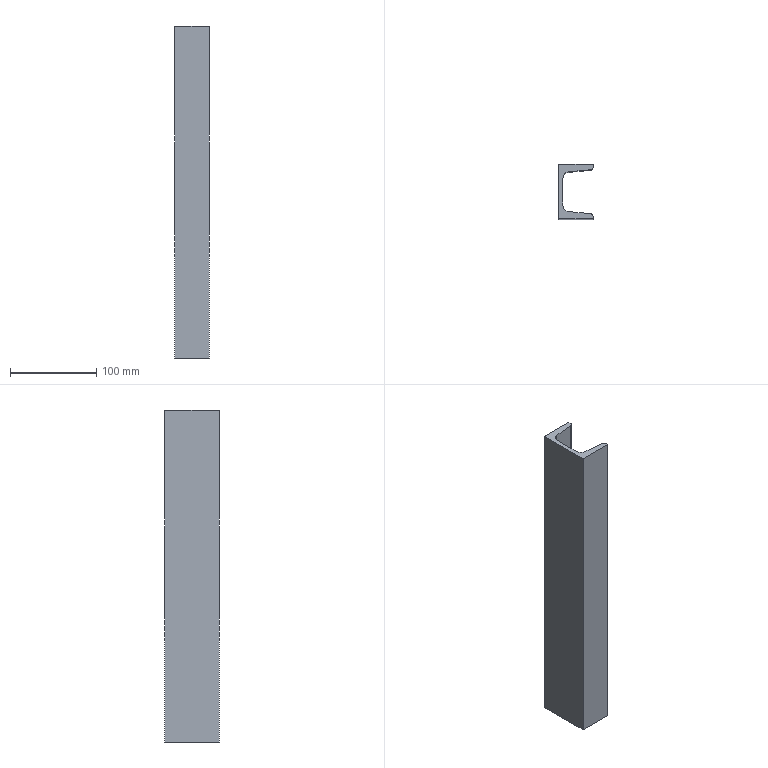Part | STEP file | 750038229 | 1 solid | 14 faces | box 40 x 63 x 384 mm | volume 324314 mm3 | plane 10 | cylinder 4 | commonest cylinder face diameters 7.6 x2 15 x2
STEP:
#1=CARTESIAN_POINT('',(0.,0.,192.));
#2=VERTEX_POINT('',#1);
#3=CARTESIAN_POINT('',(0.,0.,-192.));
#4=VERTEX_POINT('',#3);
#5=CARTESIAN_POINT('',(0.,0.,192.));
#6=DIRECTION('',(0.,0.,-1.));
#7=VECTOR('',#6,1000.);
#8=LINE('',#5,#7);
#9=EDGE_CURVE('',#2,#4,#8,.T.);
#10=ORIENTED_EDGE('',*,*,#9,.F.);
#11=CARTESIAN_POINT('',(0.,63.,192.));
#12=VERTEX_POINT('',#11);
#13=CARTESIAN_POINT('',(0.,63.,192.));
#14=DIRECTION('',(0.,-1.,0.));
#15=VECTOR('',#14,1000.);
#16=LINE('',#13,#15);
#17=EDGE_CURVE('',#12,#2,#16,.T.);
#18=ORIENTED_EDGE('',*,*,#17,.F.);
#19=CARTESIAN_POINT('',(0.,63.,-192.));
#20=VERTEX_POINT('',#19);
#21=CARTESIAN_POINT('',(0.,63.,192.));
#22=DIRECTION('',(0.,0.,1.));
#23=VECTOR('',#22,1000.);
#24=LINE('',#21,#23);
#25=EDGE_CURVE('',#20,#12,#24,.T.);
#26=ORIENTED_EDGE('',*,*,#25,.F.);
#27=CARTESIAN_POINT('',(0.,63.,-192.));
#28=DIRECTION('',(0.,1.,0.));
#29=VECTOR('',#28,1000.);
#30=LINE('',#27,#29);
#31=EDGE_CURVE('',#4,#20,#30,.T.);
#32=ORIENTED_EDGE('',*,*,#31,.F.);
#33=EDGE_LOOP('',(#10,#18,#26,#32));
#34=FACE_OUTER_BOUND('',#33,.T.);
#35=CARTESIAN_POINT('',(0.,63.,192.));
#36=DIRECTION('',(1.,0.,0.));
#37=DIRECTION('',(0.,0.,-1.));
#38=AXIS2_PLACEMENT_3D('',#35,#36,#37);
#39=PLANE('',#38);
#40=ADVANCED_FACE('',(#34),#39,.F.);
#41=CARTESIAN_POINT('',(40.,63.,-192.));
#42=VERTEX_POINT('',#41);
#43=CARTESIAN_POINT('',(36.2,63.,-192.));
#44=DIRECTION('',(-1.,0.,0.));
#45=VECTOR('',#44,1000.);
#46=LINE('',#43,#45);
#47=EDGE_CURVE('',#42,#20,#46,.T.);
#48=ORIENTED_EDGE('',*,*,#47,.F.);
#49=CARTESIAN_POINT('',(40.,60.699,-192.));
#50=VERTEX_POINT('',#49);
#51=CARTESIAN_POINT('',(40.,2.301,-192.));
#52=DIRECTION('',(0.,1.,0.));
#53=VECTOR('',#52,1000.);
#54=LINE('',#51,#53);
#55=EDGE_CURVE('',#50,#42,#54,.T.);
#56=ORIENTED_EDGE('',*,*,#55,.F.);
#57=CARTESIAN_POINT('',(36.578,56.918,-192.));
#58=VERTEX_POINT('',#57);
#59=CARTESIAN_POINT('',(36.2,60.699,-192.));
#60=DIRECTION('',(0.,0.,1.));
#61=DIRECTION('',(-1.,0.,0.));
#62=AXIS2_PLACEMENT_3D('',#59,#60,#61);
#63=CIRCLE('',#62,3.8);
#64=EDGE_CURVE('',#58,#50,#63,.T.);
#65=ORIENTED_EDGE('',*,*,#64,.F.);
#66=CARTESIAN_POINT('',(11.554,54.415,-192.));
#67=VERTEX_POINT('',#66);
#68=CARTESIAN_POINT('',(11.554,54.415,-192.));
#69=DIRECTION('',(0.995,0.0995,0.));
#70=VECTOR('',#69,1000.);
#71=LINE('',#68,#70);
#72=EDGE_CURVE('',#67,#58,#71,.T.);
#73=ORIENTED_EDGE('',*,*,#72,.F.);
#74=CARTESIAN_POINT('',(4.8,46.953,-192.));
#75=VERTEX_POINT('',#74);
#76=CARTESIAN_POINT('',(12.3,46.953,-192.));
#77=DIRECTION('',(0.,0.,-1.));
#78=DIRECTION('',(-1.,0.,0.));
#79=AXIS2_PLACEMENT_3D('',#76,#77,#78);
#80=CIRCLE('',#79,7.5);
#81=EDGE_CURVE('',#75,#67,#80,.T.);
#82=ORIENTED_EDGE('',*,*,#81,.F.);
#83=CARTESIAN_POINT('',(4.8,16.047,-192.));
#84=VERTEX_POINT('',#83);
#85=CARTESIAN_POINT('',(4.8,2.301,-192.));
#86=DIRECTION('',(0.,1.,0.));
#87=VECTOR('',#86,1000.);
#88=LINE('',#85,#87);
#89=EDGE_CURVE('',#84,#75,#88,.T.);
#90=ORIENTED_EDGE('',*,*,#89,.F.);
#91=CARTESIAN_POINT('',(11.554,8.585,-192.));
#92=VERTEX_POINT('',#91);
#93=CARTESIAN_POINT('',(12.3,16.047,-192.));
#94=DIRECTION('',(0.,0.,-1.));
#95=DIRECTION('',(-1.,0.,0.));
#96=AXIS2_PLACEMENT_3D('',#93,#94,#95);
#97=CIRCLE('',#96,7.5);
#98=EDGE_CURVE('',#92,#84,#97,.T.);
#99=ORIENTED_EDGE('',*,*,#98,.F.);
#100=CARTESIAN_POINT('',(36.578,6.082,-192.));
#101=VERTEX_POINT('',#100);
#102=CARTESIAN_POINT('',(36.578,6.082,-192.));
#103=DIRECTION('',(-0.995,0.0995,0.));
#104=VECTOR('',#103,1000.);
#105=LINE('',#102,#104);
#106=EDGE_CURVE('',#101,#92,#105,.T.);
#107=ORIENTED_EDGE('',*,*,#106,.F.);
#108=CARTESIAN_POINT('',(40.,2.301,-192.));
#109=VERTEX_POINT('',#108);
#110=CARTESIAN_POINT('',(36.2,2.301,-192.));
#111=DIRECTION('',(0.,0.,1.));
#112=DIRECTION('',(-1.,0.,0.));
#113=AXIS2_PLACEMENT_3D('',#110,#111,#112);
#114=CIRCLE('',#113,3.8);
#115=EDGE_CURVE('',#109,#101,#114,.T.);
#116=ORIENTED_EDGE('',*,*,#115,.F.);
#117=CARTESIAN_POINT('',(40.,0.,-192.));
#118=VERTEX_POINT('',#117);
#119=CARTESIAN_POINT('',(40.,2.301,-192.));
#120=DIRECTION('',(0.,1.,0.));
#121=VECTOR('',#120,1000.);
#122=LINE('',#119,#121);
#123=EDGE_CURVE('',#118,#109,#122,.T.);
#124=ORIENTED_EDGE('',*,*,#123,.F.);
#125=CARTESIAN_POINT('',(36.2,0.,-192.));
#126=DIRECTION('',(1.,0.,0.));
#127=VECTOR('',#126,1000.);
#128=LINE('',#125,#127);
#129=EDGE_CURVE('',#4,#118,#128,.T.);
#130=ORIENTED_EDGE('',*,*,#129,.F.);
#131=ORIENTED_EDGE('',*,*,#31,.T.);
#132=EDGE_LOOP('',(#48,#56,#65,#73,#82,#90,#99,#107,#116,#124,#130,#131));
#133=FACE_OUTER_BOUND('',#132,.T.);
#134=CARTESIAN_POINT('',(36.2,2.301,-192.));
#135=DIRECTION('',(0.,0.,1.));
#136=DIRECTION('',(1.,0.,0.));
#137=AXIS2_PLACEMENT_3D('',#134,#135,#136);
#138=PLANE('',#137);
#139=ADVANCED_FACE('',(#133),#138,.F.);
#140=CARTESIAN_POINT('',(40.,0.,192.));
#141=VERTEX_POINT('',#140);
#142=CARTESIAN_POINT('',(40.,0.,192.));
#143=DIRECTION('',(0.,0.,-1.));
#144=VECTOR('',#143,1000.);
#145=LINE('',#142,#144);
#146=EDGE_CURVE('',#141,#118,#145,.T.);
#147=ORIENTED_EDGE('',*,*,#146,.F.);
#148=CARTESIAN_POINT('',(0.,0.,192.));
#149=DIRECTION('',(1.,0.,0.));
#150=VECTOR('',#149,1000.);
#151=LINE('',#148,#150);
#152=EDGE_CURVE('',#2,#141,#151,.T.);
#153=ORIENTED_EDGE('',*,*,#152,.F.);
#154=ORIENTED_EDGE('',*,*,#9,.T.);
#155=ORIENTED_EDGE('',*,*,#129,.T.);
#156=EDGE_LOOP('',(#147,#153,#154,#155));
#157=FACE_OUTER_BOUND('',#156,.T.);
#158=CARTESIAN_POINT('',(0.,0.,192.));
#159=DIRECTION('',(0.,1.,0.));
#160=DIRECTION('',(0.,0.,1.));
#161=AXIS2_PLACEMENT_3D('',#158,#159,#160);
#162=PLANE('',#161);
#163=ADVANCED_FACE('',(#157),#162,.F.);
#164=CARTESIAN_POINT('',(40.,60.699,192.));
#165=VERTEX_POINT('',#164);
#166=CARTESIAN_POINT('',(40.,63.,192.));
#167=VERTEX_POINT('',#166);
#168=CARTESIAN_POINT('',(40.,2.301,192.));
#169=DIRECTION('',(0.,1.,0.));
#170=VECTOR('',#169,1000.);
#171=LINE('',#168,#170);
#172=EDGE_CURVE('',#165,#167,#171,.T.);
#173=ORIENTED_EDGE('',*,*,#172,.T.);
#174=CARTESIAN_POINT('',(36.2,63.,192.));
#175=DIRECTION('',(-1.,0.,0.));
#176=VECTOR('',#175,1000.);
#177=LINE('',#174,#176);
#178=EDGE_CURVE('',#167,#12,#177,.T.);
#179=ORIENTED_EDGE('',*,*,#178,.T.);
#180=ORIENTED_EDGE('',*,*,#17,.T.);
#181=ORIENTED_EDGE('',*,*,#152,.T.);
#182=CARTESIAN_POINT('',(40.,2.301,192.));
#183=VERTEX_POINT('',#182);
#184=CARTESIAN_POINT('',(40.,2.301,192.));
#185=DIRECTION('',(0.,1.,0.));
#186=VECTOR('',#185,1000.);
#187=LINE('',#184,#186);
#188=EDGE_CURVE('',#141,#183,#187,.T.);
#189=ORIENTED_EDGE('',*,*,#188,.T.);
#190=CARTESIAN_POINT('',(36.578,6.082,192.));
#191=VERTEX_POINT('',#190);
#192=CARTESIAN_POINT('',(36.2,2.301,192.));
#193=DIRECTION('',(0.,0.,1.));
#194=DIRECTION('',(-1.,0.,0.));
#195=AXIS2_PLACEMENT_3D('',#192,#193,#194);
#196=CIRCLE('',#195,3.8);
#197=EDGE_CURVE('',#183,#191,#196,.T.);
#198=ORIENTED_EDGE('',*,*,#197,.T.);
#199=CARTESIAN_POINT('',(11.554,8.585,192.));
#200=VERTEX_POINT('',#199);
#201=CARTESIAN_POINT('',(36.578,6.082,192.));
#202=DIRECTION('',(-0.995,0.0995,0.));
#203=VECTOR('',#202,1000.);
#204=LINE('',#201,#203);
#205=EDGE_CURVE('',#191,#200,#204,.T.);
#206=ORIENTED_EDGE('',*,*,#205,.T.);
#207=CARTESIAN_POINT('',(4.8,16.047,192.));
#208=VERTEX_POINT('',#207);
#209=CARTESIAN_POINT('',(12.3,16.047,192.));
#210=DIRECTION('',(0.,0.,-1.));
#211=DIRECTION('',(-1.,0.,0.));
#212=AXIS2_PLACEMENT_3D('',#209,#210,#211);
#213=CIRCLE('',#212,7.5);
#214=EDGE_CURVE('',#200,#208,#213,.T.);
#215=ORIENTED_EDGE('',*,*,#214,.T.);
#216=CARTESIAN_POINT('',(4.8,46.953,192.));
#217=VERTEX_POINT('',#216);
#218=CARTESIAN_POINT('',(4.8,2.301,192.));
#219=DIRECTION('',(0.,1.,0.));
#220=VECTOR('',#219,1000.);
#221=LINE('',#218,#220);
#222=EDGE_CURVE('',#208,#217,#221,.T.);
#223=ORIENTED_EDGE('',*,*,#222,.T.);
#224=CARTESIAN_POINT('',(11.554,54.415,192.));
#225=VERTEX_POINT('',#224);
#226=CARTESIAN_POINT('',(12.3,46.953,192.));
#227=DIRECTION('',(0.,0.,-1.));
#228=DIRECTION('',(-1.,0.,0.));
#229=AXIS2_PLACEMENT_3D('',#226,#227,#228);
#230=CIRCLE('',#229,7.5);
#231=EDGE_CURVE('',#217,#225,#230,.T.);
#232=ORIENTED_EDGE('',*,*,#231,.T.);
#233=CARTESIAN_POINT('',(36.578,56.918,192.));
#234=VERTEX_POINT('',#233);
#235=CARTESIAN_POINT('',(11.554,54.415,192.));
#236=DIRECTION('',(0.995,0.0995,0.));
#237=VECTOR('',#236,1000.);
#238=LINE('',#235,#237);
#239=EDGE_CURVE('',#225,#234,#238,.T.);
#240=ORIENTED_EDGE('',*,*,#239,.T.);
#241=CARTESIAN_POINT('',(36.2,60.699,192.));
#242=DIRECTION('',(0.,0.,1.));
#243=DIRECTION('',(-1.,0.,0.));
#244=AXIS2_PLACEMENT_3D('',#241,#242,#243);
#245=CIRCLE('',#244,3.8);
#246=EDGE_CURVE('',#234,#165,#245,.T.);
#247=ORIENTED_EDGE('',*,*,#246,.T.);
#248=EDGE_LOOP('',(#173,#179,#180,#181,#189,#198,#206,#215,#223,#232,#240,#247));
#249=FACE_OUTER_BOUND('',#248,.T.);
#250=CARTESIAN_POINT('',(36.2,2.301,192.));
#251=DIRECTION('',(0.,0.,1.));
#252=DIRECTION('',(1.,0.,0.));
#253=AXIS2_PLACEMENT_3D('',#250,#251,#252);
#254=PLANE('',#253);
#255=ADVANCED_FACE('',(#249),#254,.T.);
#256=ORIENTED_EDGE('',*,*,#25,.T.);
#257=ORIENTED_EDGE('',*,*,#178,.F.);
#258=CARTESIAN_POINT('',(40.,63.,192.));
#259=DIRECTION('',(0.,0.,1.));
#260=VECTOR('',#259,1000.);
#261=LINE('',#258,#260);
#262=EDGE_CURVE('',#42,#167,#261,.T.);
#263=ORIENTED_EDGE('',*,*,#262,.F.);
#264=ORIENTED_EDGE('',*,*,#47,.T.);
#265=EDGE_LOOP('',(#256,#257,#263,#264));
#266=FACE_OUTER_BOUND('',#265,.T.);
#267=CARTESIAN_POINT('',(40.,63.,192.));
#268=DIRECTION('',(0.,-1.,0.));
#269=DIRECTION('',(0.,0.,-1.));
#270=AXIS2_PLACEMENT_3D('',#267,#268,#269);
#271=PLANE('',#270);
#272=ADVANCED_FACE('',(#266),#271,.F.);
#273=ORIENTED_EDGE('',*,*,#262,.T.);
#274=ORIENTED_EDGE('',*,*,#172,.F.);
#275=CARTESIAN_POINT('',(40.,60.699,192.));
#276=DIRECTION('',(0.,0.,1.));
#277=VECTOR('',#276,1000.);
#278=LINE('',#275,#277);
#279=EDGE_CURVE('',#50,#165,#278,.T.);
#280=ORIENTED_EDGE('',*,*,#279,.F.);
#281=ORIENTED_EDGE('',*,*,#55,.T.);
#282=EDGE_LOOP('',(#273,#274,#280,#281));
#283=FACE_OUTER_BOUND('',#282,.T.);
#284=CARTESIAN_POINT('',(40.,60.699,192.));
#285=DIRECTION('',(-1.,0.,0.));
#286=DIRECTION('',(0.,-1.,0.));
#287=AXIS2_PLACEMENT_3D('',#284,#285,#286);
#288=PLANE('',#287);
#289=ADVANCED_FACE('',(#283),#288,.F.);
#290=ORIENTED_EDGE('',*,*,#246,.F.);
#291=CARTESIAN_POINT('',(36.578,56.918,192.));
#292=DIRECTION('',(0.,0.,-1.));
#293=VECTOR('',#292,1000.);
#294=LINE('',#291,#293);
#295=EDGE_CURVE('',#234,#58,#294,.T.);
#296=ORIENTED_EDGE('',*,*,#295,.T.);
#297=ORIENTED_EDGE('',*,*,#64,.T.);
#298=ORIENTED_EDGE('',*,*,#279,.T.);
#299=EDGE_LOOP('',(#290,#296,#297,#298));
#300=FACE_OUTER_BOUND('',#299,.T.);
#301=CARTESIAN_POINT('',(36.2,60.699,192.));
#302=DIRECTION('',(0.,0.,-1.));
#303=DIRECTION('',(-1.,0.,0.));
#304=AXIS2_PLACEMENT_3D('',#301,#302,#303);
#305=CYLINDRICAL_SURFACE('',#304,3.8);
#306=ADVANCED_FACE('',(#300),#305,.T.);
#307=ORIENTED_EDGE('',*,*,#295,.F.);
#308=ORIENTED_EDGE('',*,*,#239,.F.);
#309=CARTESIAN_POINT('',(11.554,54.415,192.));
#310=DIRECTION('',(0.,0.,1.));
#311=VECTOR('',#310,1000.);
#312=LINE('',#309,#311);
#313=EDGE_CURVE('',#67,#225,#312,.T.);
#314=ORIENTED_EDGE('',*,*,#313,.F.);
#315=ORIENTED_EDGE('',*,*,#72,.T.);
#316=EDGE_LOOP('',(#307,#308,#314,#315));
#317=FACE_OUTER_BOUND('',#316,.T.);
#318=CARTESIAN_POINT('',(11.554,54.415,192.));
#319=DIRECTION('',(-0.0995,0.995,0.));
#320=DIRECTION('',(-0.995,-0.0995,0.));
#321=AXIS2_PLACEMENT_3D('',#318,#319,#320);
#322=PLANE('',#321);
#323=ADVANCED_FACE('',(#317),#322,.F.);
#324=ORIENTED_EDGE('',*,*,#313,.T.);
#325=ORIENTED_EDGE('',*,*,#231,.F.);
#326=CARTESIAN_POINT('',(4.8,46.953,192.));
#327=DIRECTION('',(0.,0.,1.));
#328=VECTOR('',#327,1000.);
#329=LINE('',#326,#328);
#330=EDGE_CURVE('',#75,#217,#329,.T.);
#331=ORIENTED_EDGE('',*,*,#330,.F.);
#332=ORIENTED_EDGE('',*,*,#81,.T.);
#333=EDGE_LOOP('',(#324,#325,#331,#332));
#334=FACE_OUTER_BOUND('',#333,.T.);
#335=CARTESIAN_POINT('',(12.3,46.953,192.));
#336=DIRECTION('',(0.,0.,-1.));
#337=DIRECTION('',(-1.,0.,0.));
#338=AXIS2_PLACEMENT_3D('',#335,#336,#337);
#339=CYLINDRICAL_SURFACE('',#338,7.5);
#340=ADVANCED_FACE('',(#334),#339,.F.);
#341=ORIENTED_EDGE('',*,*,#330,.T.);
#342=ORIENTED_EDGE('',*,*,#222,.F.);
#343=CARTESIAN_POINT('',(4.8,16.047,192.));
#344=DIRECTION('',(0.,0.,1.));
#345=VECTOR('',#344,1000.);
#346=LINE('',#343,#345);
#347=EDGE_CURVE('',#84,#208,#346,.T.);
#348=ORIENTED_EDGE('',*,*,#347,.F.);
#349=ORIENTED_EDGE('',*,*,#89,.T.);
#350=EDGE_LOOP('',(#341,#342,#348,#349));
#351=FACE_OUTER_BOUND('',#350,.T.);
#352=CARTESIAN_POINT('',(4.8,16.047,192.));
#353=DIRECTION('',(-1.,0.,0.));
#354=DIRECTION('',(0.,-1.,0.));
#355=AXIS2_PLACEMENT_3D('',#352,#353,#354);
#356=PLANE('',#355);
#357=ADVANCED_FACE('',(#351),#356,.F.);
#358=ORIENTED_EDGE('',*,*,#347,.T.);
#359=ORIENTED_EDGE('',*,*,#214,.F.);
#360=CARTESIAN_POINT('',(11.554,8.585,192.));
#361=DIRECTION('',(0.,0.,1.));
#362=VECTOR('',#361,1000.);
#363=LINE('',#360,#362);
#364=EDGE_CURVE('',#92,#200,#363,.T.);
#365=ORIENTED_EDGE('',*,*,#364,.F.);
#366=ORIENTED_EDGE('',*,*,#98,.T.);
#367=EDGE_LOOP('',(#358,#359,#365,#366));
#368=FACE_OUTER_BOUND('',#367,.T.);
#369=CARTESIAN_POINT('',(12.3,16.047,192.));
#370=DIRECTION('',(0.,0.,-1.));
#371=DIRECTION('',(-1.,0.,0.));
#372=AXIS2_PLACEMENT_3D('',#369,#370,#371);
#373=CYLINDRICAL_SURFACE('',#372,7.5);
#374=ADVANCED_FACE('',(#368),#373,.F.);
#375=ORIENTED_EDGE('',*,*,#364,.T.);
#376=ORIENTED_EDGE('',*,*,#205,.F.);
#377=CARTESIAN_POINT('',(36.578,6.082,192.));
#378=DIRECTION('',(0.,0.,1.));
#379=VECTOR('',#378,1000.);
#380=LINE('',#377,#379);
#381=EDGE_CURVE('',#101,#191,#380,.T.);
#382=ORIENTED_EDGE('',*,*,#381,.F.);
#383=ORIENTED_EDGE('',*,*,#106,.T.);
#384=EDGE_LOOP('',(#375,#376,#382,#383));
#385=FACE_OUTER_BOUND('',#384,.T.);
#386=CARTESIAN_POINT('',(36.578,6.082,192.));
#387=DIRECTION('',(-0.0995,-0.995,0.));
#388=DIRECTION('',(0.995,-0.0995,0.));
#389=AXIS2_PLACEMENT_3D('',#386,#387,#388);
#390=PLANE('',#389);
#391=ADVANCED_FACE('',(#385),#390,.F.);
#392=ORIENTED_EDGE('',*,*,#197,.F.);
#393=CARTESIAN_POINT('',(40.,2.301,192.));
#394=DIRECTION('',(0.,0.,-1.));
#395=VECTOR('',#394,1000.);
#396=LINE('',#393,#395);
#397=EDGE_CURVE('',#183,#109,#396,.T.);
#398=ORIENTED_EDGE('',*,*,#397,.T.);
#399=ORIENTED_EDGE('',*,*,#115,.T.);
#400=ORIENTED_EDGE('',*,*,#381,.T.);
#401=EDGE_LOOP('',(#392,#398,#399,#400));
#402=FACE_OUTER_BOUND('',#401,.T.);
#403=CARTESIAN_POINT('',(36.2,2.301,192.));
#404=DIRECTION('',(0.,0.,-1.));
#405=DIRECTION('',(-1.,0.,0.));
#406=AXIS2_PLACEMENT_3D('',#403,#404,#405);
#407=CYLINDRICAL_SURFACE('',#406,3.8);
#408=ADVANCED_FACE('',(#402),#407,.T.);
#409=ORIENTED_EDGE('',*,*,#397,.F.);
#410=ORIENTED_EDGE('',*,*,#188,.F.);
#411=ORIENTED_EDGE('',*,*,#146,.T.);
#412=ORIENTED_EDGE('',*,*,#123,.T.);
#413=EDGE_LOOP('',(#409,#410,#411,#412));
#414=FACE_OUTER_BOUND('',#413,.T.);
#415=CARTESIAN_POINT('',(40.,0.,192.));
#416=DIRECTION('',(-1.,0.,0.));
#417=DIRECTION('',(0.,0.,1.));
#418=AXIS2_PLACEMENT_3D('',#415,#416,#417);
#419=PLANE('',#418);
#420=ADVANCED_FACE('',(#414),#419,.F.);
#421=CLOSED_SHELL('',(#40,#139,#163,#255,#272,#289,#306,#323,#340,#357,#374,#391,#408,#420));
#422=MANIFOLD_SOLID_BREP('',#421);
#423=CARTESIAN_POINT('',(0.,0.,0.));
#424=DIRECTION('',(0.,0.,1.));
#425=DIRECTION('',(1.,0.,0.));
#426=AXIS2_PLACEMENT_3D('',#423,#424,#425);
#427=(LENGTH_UNIT()NAMED_UNIT(*)SI_UNIT(.MILLI.,.METRE.));
#428=UNCERTAINTY_MEASURE_WITH_UNIT(LENGTH_MEASURE(0.00001),#427,'','');
#429=(NAMED_UNIT(*)PLANE_ANGLE_UNIT()SI_UNIT($,.RADIAN.));
#430=(NAMED_UNIT(*)SI_UNIT($,.STERADIAN.)SOLID_ANGLE_UNIT());
#431=(GEOMETRIC_REPRESENTATION_CONTEXT(3)GLOBAL_UNCERTAINTY_ASSIGNED_CONTEXT((#428))GLOBAL_UNIT_ASSIGNED_CONTEXT((#427,#429,#430))REPRESENTATION_CONTEXT('',''));
#432=ADVANCED_BREP_SHAPE_REPRESENTATION('',(#422,#426),#431);